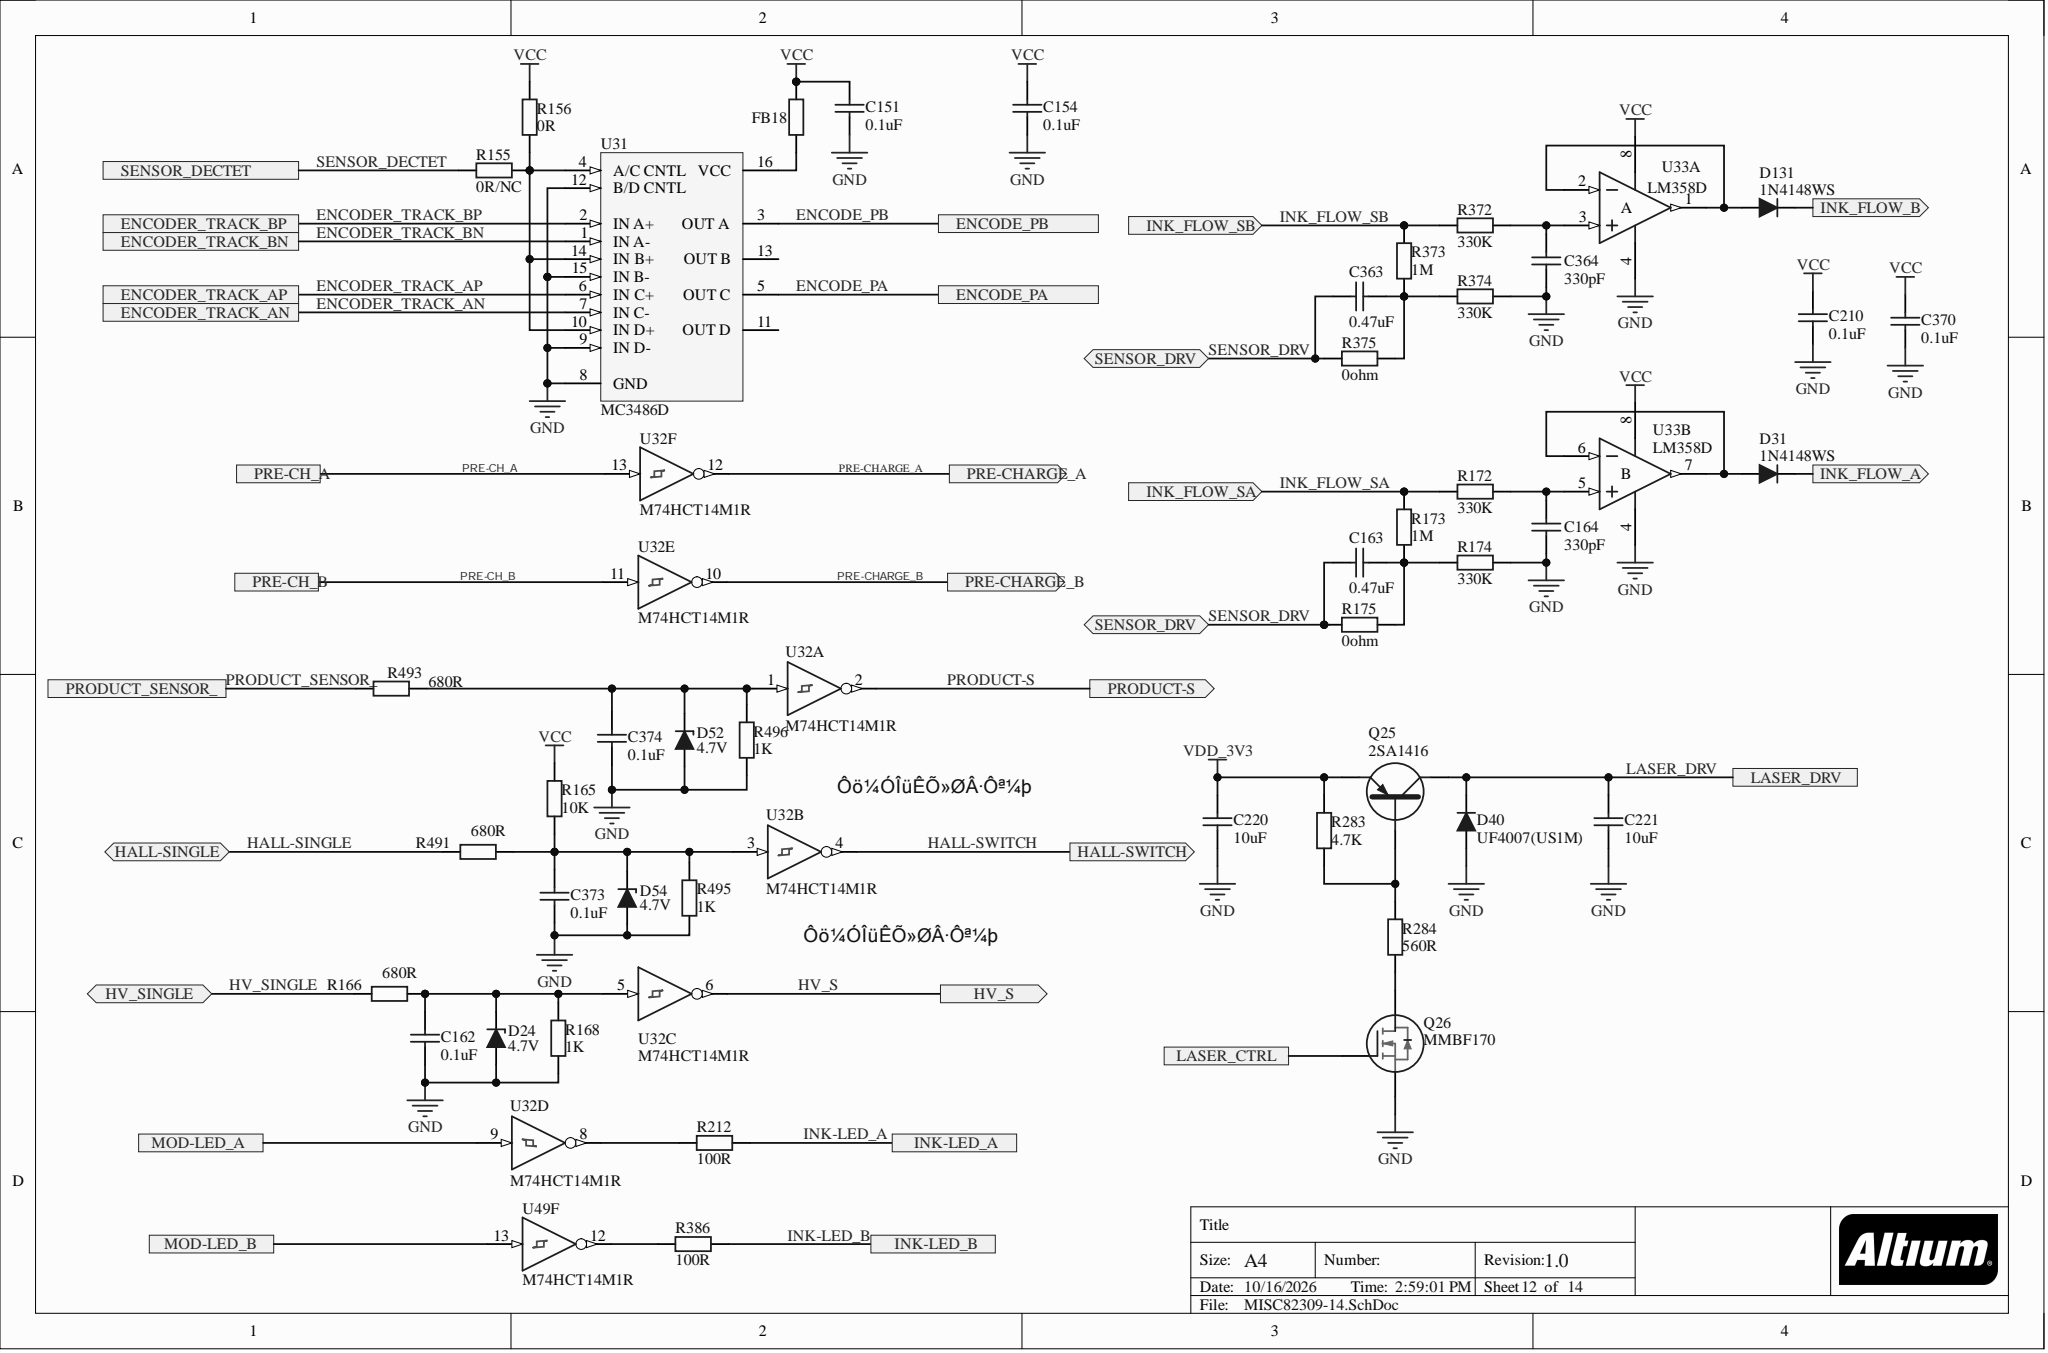Circuit board | Altium Designer | 747 parts | 576 nets | one sheet of the schematic
Parts on this sheet (reference | value | footprint):
C151 | 0.1uF | CAP_0805
C154 | 0.1uF | CAP_0805
C162 | 0.1uF | CAP_0805
C163 | 0.47uF | C0603
C164 | 330pF | C0603
C210 | 0.1uF | CAP_0603
C220 | 10uF | CAP_0805
C221 | 10uF | CAP_0805
C363 | 0.47uF | C0603
C364 | 330pF | C0603
C370 | 0.1uF | CAP_0603
C373 | 0.1uF | CAP_0805
C374 | 0.1uF | CAP_0805
D24 | 4.7V | SOD-123
D31 | 1N4148WS | SOD323
D40 | UF4007(US1M) | DO-214AA
D52 | 4.7V | SOD-123
D54 | 4.7V | SOD-123
D131 | 1N4148WS | SOD323
FB18 | 60 | SMD0805-L
Q25 | 2SA1416 | SOT89
Q26 | MMBF170 | SOT-23
R155 | 0R/NC | R0805
R156 | 0R | R0805
R165 | 10K | R0805
R166 | 680R | R0805
R168 | 1K | R0805
R172 | 330K | R0603
R173 | 1M | R0603
R174 | 330K | R0603
R175 | 0ohm | R0603
R212 | 100R | R0805
R283 | 4.7K | R0805
R284 | 560R | R0805
R372 | 330K | R0603
R373 | 1M | R0603
R374 | 330K | R0603
R375 | 0ohm | R0603
R386 | 100R | R0805
R491 | 680R | R0805
R493 | 680R | R0805
R495 | 1K | R0805
R496 | 1K | R0805
U31 | MC3486D | 751B-03
Nets of these parts (net: part-pin ...):
VDD_3V3: C220-2 Q25-3 R283-2
VCC: C151-2 C154-2 C210-2 C370-2 FB18-2 R156-2 R165-2
SENSOR_DRV: C163-2 C363-2 R175-1 R375-1
SENSOR_DECTET: R155-1
PRODUCT_SENSOR_: R493-1
NetR386_1: R386-1
NetR212_1: R212-1
NetR155_2: R155-2 R156-1 U31-4 U31-10 U31-14
NetQ26_3: Q26-3 R284-1
NetQ25_1: Q25-1 R283-1 R284-2
NetFB18_1: FB18-1 U31-16
NetD131_1: D131-1
NetD31_1: D31-1
NetC374_2: C374-2 D52-2 R493-2 R496-2
NetC373_2: C373-2 D54-2 R165-1 R491-2 R495-2
NetC364_2: C364-2 R372-1
NetC363_1: C363-1 R373-1 R374-1 R375-2
NetC164_2: C164-2 R172-1
NetC163_1: C163-1 R173-1 R174-1 R175-2
NetC162_2: C162-2 D24-2 R166-2 R168-2
LASER_DRV: C221-2 D40-2 Q25-2
LASER_CTRL: Q26-1
INK_FLOW_SB: R372-2 R373-2
INK_FLOW_SA: R172-2 R173-2
INK_FLOW_B: D131-2
INK_FLOW_A: D31-2
INK-LED_B: R386-2
INK-LED_A: R212-2
HV_SINGLE: R166-1
HALL-SINGLE: R491-1
GND: C151-1 C154-1 C162-1 C164-1 C210-1 C220-1 C221-1 C364-1 C370-1 C373-1 C374-1 D24-1 D40-1 D52-1 D54-1 Q26-2 R168-1 R174-2 R374-2 R495-1 R496-1 U31-8 U31-9 U31-12 U31-15
ENCODER_TRACK_BP: U31-2
ENCODER_TRACK_BN: U31-1
ENCODER_TRACK_AP: U31-6
ENCODER_TRACK_AN: U31-7
ENCODE_PB: U31-3
ENCODE_PA: U31-5